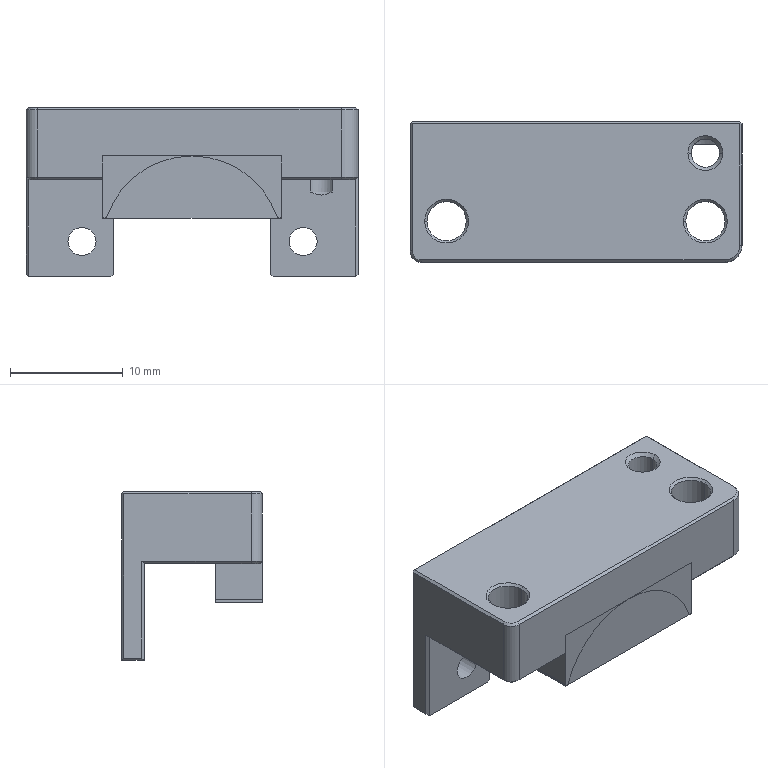NC program | NX | posted with a generic post | part box 29.5 x 12.5 x 15 mm
Whole program:
N10 G17 G21 G94 G90
(FLOOR_WALL_COPY_COPY , TOOL : D63)
N12 T03 M6
N14 G54
N16 G17 G0 G90 X-49.249 Y0. B0. C0. S6500 M3
N18 G43 Z30. H3
N20 Z7.
N22 G94 G1 Z4. F1250.
N24 X-46.249
N26 X46.249
N28 X49.249
N30 Z7.
N32 G0 Z30.
N34 X-49.249
N36 Z6.
N38 G1 Z3.
N40 X-46.249
N42 X46.249
N44 X49.249
N46 Z6.
N48 G0 Z30.
N50 X-49.249
N52 Z5.
N54 G1 Z2.
N56 X-46.249
N58 X46.249
N60 X49.249
N62 Z5.
N64 G0 Z30.
N66 X-49.249
N68 Z4.
N70 G1 Z1.
N72 X-46.249
N74 X46.249
N76 X49.249
N78 Z4.
N80 G0 Z30.
N82 X-49.249
N84 Z3.
N86 G1 Z0.
N88 X-46.249
N90 X46.249
N92 X49.249
N94 Z3.
N96 G0 Z30.
N98 M5
(FLOOR_WALL , TOOL : D6JING)
N100 T16 M6
N102 G54
N104 G17 G0 G90 X2.078 Y-12.25 B0. C0. S9500 M3
N106 G43 Z30. H16
N108 Z-0.443
N110 G94 G1 X0.52 Y-9.55 F1000.
N112 G3 X0. Y-9.25 R0.6
N114 G1 X-10.95 F2500.
N116 Y-9.05
N118 X-13.25
N120 G2 X-17.55 Y-4.75 R4.3
N122 G1 Y2.866
N124 X-15.834 Y1.15
N126 X-3.9
N128 Y9.25
N130 X3.9
N132 Y1.15
N134 X15.834
N136 X17.55 Y2.866
N138 Y-5.25
N140 G2 X13.75 Y-9.05 R3.8
N142 G1 X10.95
N144 Y-9.25
N146 X0.
N148 Y-6.25
N150 X-9.873
N152 G3 X-10.95 Y-6.05 R3.
N154 G1 X-13.25
N156 G2 X-14.55 Y-4.75 R1.3
N158 G1 Y-1.85
N160 X-3.9
N162 G3 X-0.9 Y1.15 R3.
N164 G1 Y6.25
N166 X0.9
N168 Y1.15
N170 G3 X3.9 Y-1.85 R3.
N172 G1 X14.55
N174 Y-5.25
N176 G2 X13.75 Y-6.05 R0.8
N178 G1 X10.95
N180 G3 X9.873 Y-6.25 R3.
N182 G1 X0.
N184 Y-3.55
N186 X-0.675
N188 G3 X0. Y-3.007 R5.7
N190 X0.675 Y-3.55 R5.7
N192 G1 X0.
N194 G3 X-0.52 Y-3.85 R0.6
N196 G1 Y-12.25
N198 G0 X2.078 Z-0.906
N200 G1 X0.52 Y-9.55 F1000.
N202 G3 X0. Y-9.25 R0.6
N204 G1 X-10.95 F2500.
N206 Y-9.05
N208 X-13.25
N210 G2 X-17.55 Y-4.75 R4.3
N212 G1 Y2.866
N214 X-15.834 Y1.15
N216 X-3.9
N218 Y9.25
N220 X3.9
N222 Y1.15
N224 X15.834
N226 X17.55 Y2.866
N228 Y-5.25
N230 G2 X13.75 Y-9.05 R3.8
N232 G1 X10.95
N234 Y-9.25
N236 X0.
N238 Y-6.25
N240 X-9.873
N242 G3 X-10.95 Y-6.05 R3.
N244 G1 X-13.25
N246 G2 X-14.55 Y-4.75 R1.3
N248 G1 Y-1.85
N250 X-3.9
N252 G3 X-0.9 Y1.15 R3.
N254 G1 Y6.25
N256 X0.9
N258 Y1.15
N260 G3 X3.9 Y-1.85 R3.
N262 G1 X14.55
N264 Y-5.25
N266 G2 X13.75 Y-6.05 R0.8
N268 G1 X10.95
N270 G3 X9.873 Y-6.25 R3.
N272 G1 X0.
N274 Y-3.55
N276 X-0.675
N278 G3 X0. Y-3.007 R5.7
N280 X0.675 Y-3.55 R5.7
N282 G1 X0.
N284 G3 X-0.52 Y-3.85 R0.6
N286 G1 Y-12.25
N288 G0 X2.078 Z-1.37
N290 G1 X0.52 Y-9.55 F1000.
N292 G3 X0. Y-9.25 R0.6
N294 G1 X-10.95 F2500.
N296 Y-9.05
N298 X-13.25
N300 G2 X-17.55 Y-4.75 R4.3
N302 G1 Y2.866
N304 X-15.834 Y1.15
N306 X-3.9
N308 Y9.25
N310 X3.9
N312 Y1.15
N314 X15.834
N316 X17.55 Y2.866
N318 Y-5.25
N320 G2 X13.75 Y-9.05 R3.8
N322 G1 X10.95
N324 Y-9.25
N326 X0.
N328 Y-6.25
N330 X-9.873
N332 G3 X-10.95 Y-6.05 R3.
N334 G1 X-13.25
N336 G2 X-14.55 Y-4.75 R1.3
N338 G1 Y-1.85
N340 X-3.9
N342 G3 X-0.9 Y1.15 R3.
N344 G1 Y6.25
N346 X0.9
N348 Y1.15
N350 G3 X3.9 Y-1.85 R3.
N352 G1 X14.55
N354 Y-5.25
N356 G2 X13.75 Y-6.05 R0.8
N358 G1 X10.95
N360 G3 X9.873 Y-6.25 R3.
N362 G1 X0.
N364 Y-3.55
N366 X-0.675
N368 G3 X0. Y-3.007 R5.7
N370 X0.675 Y-3.55 R5.7
N372 G1 X0.
N374 G3 X-0.52 Y-3.85 R0.6
N376 G1 Y-12.25
N378 G0 X2.078 Z-1.834
N380 G1 X0.52 Y-9.55 F1000.
N382 G3 X0. Y-9.25 R0.6
N384 G1 X-10.95 F2500.
N386 Y-9.05
N388 X-13.25
N390 G2 X-17.55 Y-4.75 R4.3
N392 G1 Y2.866
N394 X-15.834 Y1.15
N396 X-3.9
N398 Y9.25
N400 X3.9
N402 Y1.15
N404 X15.834
N406 X17.55 Y2.866
N408 Y-5.25
N410 G2 X13.75 Y-9.05 R3.8
N412 G1 X10.95
N414 Y-9.25
N416 X0.
N418 Y-6.25
N420 X-9.873
N422 G3 X-10.95 Y-6.05 R3.
N424 G1 X-13.25
N426 G2 X-14.55 Y-4.75 R1.3
N428 G1 Y-1.85
N430 X-3.9
N432 G3 X-0.9 Y1.15 R3.
N434 G1 Y6.25
N436 X0.9
N438 Y1.15
N440 G3 X3.9 Y-1.85 R3.
N442 G1 X14.55
N444 Y-5.25
N446 G2 X13.75 Y-6.05 R0.8
N448 G1 X10.95
N450 G3 X9.873 Y-6.25 R3.
N452 G1 X0.
N454 Y-3.55
N456 X-0.675
N458 G3 X0. Y-3.007 R5.7
N460 X0.675 Y-3.55 R5.7
N462 G1 X0.
N464 G3 X-0.52 Y-3.85 R0.6
N466 G1 Y-12.25
N468 G0 X2.078 Z-2.297
N470 G1 X0.52 Y-9.55 F1000.
N472 G3 X0. Y-9.25 R0.6
N474 G1 X-10.95 F2500.
N476 Y-9.05
N478 X-13.25
N480 G2 X-17.55 Y-4.75 R4.3
N482 G1 Y2.866
N484 X-15.834 Y1.15
N486 X-3.9
N488 Y9.25
N490 X3.9
N492 Y1.15
N494 X15.834
N496 X17.55 Y2.866
N498 Y-5.25
N500 G2 X13.75 Y-9.05 R3.8
N502 G1 X10.95
N504 Y-9.25
N506 X0.
N508 Y-6.25
N510 X-9.873
N512 G3 X-10.95 Y-6.05 R3.
N514 G1 X-13.25
N516 G2 X-14.55 Y-4.75 R1.3
N518 G1 Y-1.85
N520 X-3.9
N522 G3 X-0.9 Y1.15 R3.
N524 G1 Y6.25
N526 X0.9
N528 Y1.15
N530 G3 X3.9 Y-1.85 R3.
N532 G1 X14.55
N534 Y-5.25
N536 G2 X13.75 Y-6.05 R0.8
N538 G1 X10.95
N540 G3 X9.873 Y-6.25 R3.
N542 G1 X0.
N544 Y-3.55
N546 X-0.675
N548 G3 X0. Y-3.007 R5.7
N550 X0.675 Y-3.55 R5.7
N552 G1 X0.
N554 G3 X-0.52 Y-3.85 R0.6
N556 G1 Y-12.25
N558 G0 X2.078 Z-2.761
N560 G1 X0.52 Y-9.55 F1000.
N562 G3 X0. Y-9.25 R0.6
N564 G1 X-10.95 F2500.
N566 Y-9.05
N568 X-13.25
N570 G2 X-17.55 Y-4.75 R4.3
N572 G1 Y2.866
N574 X-15.834 Y1.15
N576 X-3.9
N578 Y9.25
N580 X3.9
N582 Y1.15
N584 X15.834
N586 X17.55 Y2.866
N588 Y-5.25
N590 G2 X13.75 Y-9.05 R3.8
N592 G1 X10.95
N594 Y-9.25
N596 X0.
N598 Y-6.25
N600 X-9.873
N602 G3 X-10.95 Y-6.05 R3.
N604 G1 X-13.25
N606 G2 X-14.55 Y-4.75 R1.3
N608 G1 Y-1.85
N610 X-3.9
N612 G3 X-0.9 Y1.15 R3.
N614 G1 Y6.25
N616 X0.9
N618 Y1.15
N620 G3 X3.9 Y-1.85 R3.
N622 G1 X14.55
N624 Y-5.25
N626 G2 X13.75 Y-6.05 R0.8
N628 G1 X10.95
N630 G3 X9.873 Y-6.25 R3.
N632 G1 X0.
N634 Y-3.55
N636 X-0.675
N638 G3 X0. Y-3.007 R5.7
N640 X0.675 Y-3.55 R5.7
N642 G1 X0.
N644 G3 X-0.52 Y-3.85 R0.6
N646 G1 Y-12.25
N648 G0 X2.078 Z-3.225
N650 G1 X0.52 Y-9.55 F1000.
N652 G3 X0. Y-9.25 R0.6
N654 G1 X-10.95 F2500.
N656 Y-9.05
N658 X-13.25
N660 G2 X-17.55 Y-4.75 R4.3
N662 G1 Y2.866
N664 X-15.834 Y1.15
N666 X-3.9
N668 Y9.25
N670 X3.9
N672 Y1.15
N674 X15.834
N676 X17.55 Y2.866
N678 Y-5.25
N680 G2 X13.75 Y-9.05 R3.8
N682 G1 X10.95
N684 Y-9.25
N686 X0.
N688 Y-6.25
N690 X-9.873
N692 G3 X-10.95 Y-6.05 R3.
N694 G1 X-13.25
N696 G2 X-14.55 Y-4.75 R1.3
N698 G1 Y-1.85
N700 X-3.9
N702 G3 X-0.9 Y1.15 R3.
N704 G1 Y6.25
N706 X0.9
N708 Y1.15
N710 G3 X3.9 Y-1.85 R3.
N712 G1 X14.55
N714 Y-5.25
N716 G2 X13.75 Y-6.05 R0.8
N718 G1 X10.95
N720 G3 X9.873 Y-6.25 R3.
N722 G1 X0.
N724 Y-3.55
N726 X-0.675
N728 G3 X0. Y-3.007 R5.7
N730 X0.675 Y-3.55 R5.7
N732 G1 X0.
N734 G3 X-0.52 Y-3.85 R0.6
N736 G1 Y-12.25
N738 G0 X2.078 Z-3.688
N740 G1 X0.52 Y-9.55 F1000.
N742 G3 X0. Y-9.25 R0.6
N744 G1 X-10.95 F2500.
N746 Y-9.05
N748 X-13.25
N750 G2 X-17.55 Y-4.75 R4.3
N752 G1 Y2.866
N754 X-15.834 Y1.15
N756 X-3.9
N758 Y9.25
N760 X3.9
N762 Y1.15
N764 X15.834
N766 X17.55 Y2.866
N768 Y-5.25
N770 G2 X13.75 Y-9.05 R3.8
N772 G1 X10.95
N774 Y-9.25
N776 X0.
N778 Y-6.25
N780 X-9.873
N782 G3 X-10.95 Y-6.05 R3.
N784 G1 X-13.25
N786 G2 X-14.55 Y-4.75 R1.3
N788 G1 Y-1.85
N790 X-3.9
N792 G3 X-0.9 Y1.15 R3.
N794 G1 Y6.25
N796 X0.9
N798 Y1.15
N800 G3 X3.9 Y-1.85 R3.
N802 G1 X14.55
N804 Y-5.25
N806 G2 X13.75 Y-6.05 R0.8
N808 G1 X10.95
N810 G3 X9.873 Y-6.25 R3.
N812 G1 X0.
N814 Y-3.55
N816 X-0.675
N818 G3 X0. Y-3.007 R5.7
N820 X0.675 Y-3.55 R5.7
N822 G1 X0.
N824 G3 X-0.52 Y-3.85 R0.6
N826 G1 Y-12.25
N828 G0 X2.078 Z-4.152
N830 G1 X0.52 Y-9.55 F1000.
N832 G3 X0. Y-9.25 R0.6
N834 G1 X-10.95 F2500.
N836 Y-9.05
N838 X-13.25
N840 G2 X-17.55 Y-4.75 R4.3
N842 G1 Y2.866
N844 X-15.834 Y1.15
N846 X-3.9
N848 Y9.25
N850 X3.9
N852 Y1.15
N854 X15.834
N856 X17.55 Y2.866
N858 Y-5.25
N860 G2 X13.75 Y-9.05 R3.8
N862 G1 X10.95
N864 Y-9.25
N866 X0.
N868 Y-6.25
N870 X-9.873
N872 G3 X-10.95 Y-6.05 R3.
N874 G1 X-13.25
N876 G2 X-14.55 Y-4.75 R1.3
N878 G1 Y-1.85
N880 X-3.9
N882 G3 X-0.9 Y1.15 R3.
N884 G1 Y6.25
N886 X0.9
N888 Y1.15
N890 G3 X3.9 Y-1.85 R3.
N892 G1 X14.55
N894 Y-5.25
N896 G2 X13.75 Y-6.05 R0.8
N898 G1 X10.95
N900 G3 X9.873 Y-6.25 R3.
N902 G1 X0.
N904 Y-3.55
N906 X-0.675
N908 G3 X0. Y-3.007 R5.7
N910 X0.675 Y-3.55 R5.7
N912 G1 X0.
N914 G3 X-0.52 Y-3.85 R0.6
N916 G1 Y-12.25
N918 G0 X2.078 Z-4.615
N920 G1 X0.52 Y-9.55 F1000.
N922 G3 X0. Y-9.25 R0.6
N924 G1 X-10.95 F2500.
N926 Y-9.05
N928 X-13.25
N930 G2 X-17.55 Y-4.75 R4.3
N932 G1 Y2.866
N934 X-15.834 Y1.15
N936 X-3.9
N938 Y9.25
N940 X3.9
N942 Y1.15
N944 X15.834
N946 X17.55 Y2.866
N948 Y-5.25
N950 G2 X13.75 Y-9.05 R3.8
N952 G1 X10.95
N954 Y-9.25
N956 X0.
N958 Y-6.25
N960 X-9.873
N962 G3 X-10.95 Y-6.05 R3.
N964 G1 X-13.25
N966 G2 X-14.55 Y-4.75 R1.3
N968 G1 Y-1.85
N970 X-3.9
N972 G3 X-0.9 Y1.15 R3.
N974 G1 Y6.25
N976 X0.9
N978 Y1.15
N980 G3 X3.9 Y-1.85 R3.
N982 G1 X14.55
N984 Y-5.25
N986 G2 X13.75 Y-6.05 R0.8
N988 G1 X10.95
N990 G3 X9.873 Y-6.25 R3.
N992 G1 X0.
N994 Y-3.55
N996 X-0.675
N998 G3 X0. Y-3.007 R5.7
N1000 X0.675 Y-3.55 R5.7
N1002 G1 X0.
N1004 G3 X-0.52 Y-3.85 R0.6
N1006 G1 Y-12.25
N1008 G0 X2.078 Z-5.079
N1010 G1 X0.52 Y-9.55 F1000.
N1012 G3 X0. Y-9.25 R0.6
N1014 G1 X-10.95 F2500.
N1016 Y-9.05
N1018 X-13.25
N1020 G2 X-17.55 Y-4.75 R4.3
N1022 G1 Y2.866
N1024 X-15.834 Y1.15
N1026 X-3.9
N1028 Y9.25
N1030 X3.9
N1032 Y1.15
N1034 X15.834
N1036 X17.55 Y2.866
N1038 Y-5.25
N1040 G2 X13.75 Y-9.05 R3.8
N1042 G1 X10.95
N1044 Y-9.25
N1046 X0.
N1048 Y-6.25
N1050 X-9.873
N1052 G3 X-10.95 Y-6.05 R3.
N1054 G1 X-13.25
N1056 G2 X-14.55 Y-4.75 R1.3
N1058 G1 Y-1.85
N1060 X-3.9
N1062 G3 X-0.9 Y1.15 R3.
N1064 G1 Y6.25
N1066 X0.9
N1068 Y1.15
N1070 G3 X3.9 Y-1.85 R3.
N1072 G1 X14.55
N1074 Y-5.25
N1076 G2 X13.75 Y-6.05 R0.8
N1078 G1 X10.95
N1080 G3 X9.873 Y-6.25 R3.
N1082 G1 X0.
N1084 Y-3.55
N1086 X-0.675
N1088 G3 X0. Y-3.007 R5.7
N1090 X0.675 Y-3.55 R5.7
N1092 G1 X0.
N1094 G3 X-0.52 Y-3.85 R0.6
N1096 G1 Y-12.25
N1098 G0 Z30.
N1100 X-2.136 Y12.35
N1102 Z-5.568
N1104 G1 X-0.52 Y9.55 F1000.
N1106 G3 X0. Y9.25 R0.6
N1108 G1 X3.9 F2500.
N1110 Y1.15
N1112 X15.834
N1114 X17.55 Y2.866
N1116 Y-5.25
N1118 G2 X13.75 Y-9.05 R3.8
N1120 G1 X11.05
N1122 Y-1.85
N1124 X14.05
N1126 X14.55
N1128 Y-5.25
N1130 G2 X14.05 Y-5.992 R0.8
N1132 G1 Y-1.85
N1134 X11.05
N1136 Y1.05
N1138 X-11.05
N1140 Y-9.05
N1142 X-13.25
N1144 G2 X-17.55 Y-4.75 R4.3
N1146 G1 Y2.866
N1148 X-15.834 Y1.15
N1150 X-14.05
N1152 Y-1.85
N1154 Y-5.775
N1156 G2 X-14.55 Y-4.75 R1.3
N1158 G1 Y-1.85
N1160 X-14.05
N1162 Y1.15
N1164 X-3.9
N1166 Y9.25
N1168 X0.
N1170 Y6.25
N1172 X0.9
N1174 Y4.05
N1176 X-0.9
N1178 Y6.25
N1180 X0.
N1182 G3 X0.52 Y6.55 R0.6
N1184 G1 Y12.25
N1186 G0 X-2.136 Y12.35 Z-6.056
N1188 G1 X-0.52 Y9.55 F1000.
N1190 G3 X0. Y9.25 R0.6
N1192 G1 X3.9 F2500.
N1194 Y1.15
N1196 X15.834
N1198 X17.55 Y2.866
N1200 Y-5.25
N1202 G2 X13.75 Y-9.05 R3.8
N1204 G1 X11.05
N1206 Y-1.85
N1208 X14.05
N1210 X14.55
N1212 Y-5.25
N1214 G2 X14.05 Y-5.992 R0.8
N1216 G1 Y-1.85
N1218 X11.05
N1220 Y1.05
N1222 X-11.05
N1224 Y-9.05
N1226 X-13.25
N1228 G2 X-17.55 Y-4.75 R4.3
N1230 G1 Y2.866
N1232 X-15.834 Y1.15
N1234 X-14.05
N1236 Y-1.85
N1238 Y-5.775
N1240 G2 X-14.55 Y-4.75 R1.3
N1242 G1 Y-1.85
N1244 X-14.05
N1246 Y1.15
N1248 X-3.9
N1250 Y9.25
N1252 X0.
N1254 Y6.25
N1256 X0.9
N1258 Y4.05
N1260 X-0.9
N1262 Y6.25
N1264 X0.
N1266 G3 X0.52 Y6.55 R0.6
N1268 G1 Y12.25
N1270 G0 X-2.136 Y12.35 Z-6.545
N1272 G1 X-0.52 Y9.55 F1000.
N1274 G3 X0. Y9.25 R0.6
N1276 G1 X3.9 F2500.
N1278 Y1.15
N1280 X15.834
N1282 X17.55 Y2.866
N1284 Y-5.25
N1286 G2 X13.75 Y-9.05 R3.8
N1288 G1 X11.05
N1290 Y-1.85
N1292 X14.05
N1294 X14.55
N1296 Y-5.25
N1298 G2 X14.05 Y-5.992 R0.8
N1300 G1 Y-1.85
N1302 X11.05
N1304 Y1.05
N1306 X-11.05
N1308 Y-9.05
N1310 X-13.25
N1312 G2 X-17.55 Y-4.75 R4.3
N1314 G1 Y2.866
N1316 X-15.834 Y1.15
N1318 X-14.05
N1320 Y-1.85
N1322 Y-5.775
N1324 G2 X-14.55 Y-4.75 R1.3
N1326 G1 Y-1.85
N1328 X-14.05
N1330 Y1.15
N1332 X-3.9
N1334 Y9.25
N1336 X0.
N1338 Y6.25
N1340 X0.9
N1342 Y4.05
N1344 X-0.9
N1346 Y6.25
N1348 X0.
N1350 G3 X0.52 Y6.55 R0.6
N1352 G1 Y12.25
N1354 G0 X-2.136 Y12.35 Z-7.034
N1356 G1 X-0.52 Y9.55 F1000.
N1358 G3 X0. Y9.25 R0.6
N1360 G1 X3.9 F2500.
N1362 Y1.15
N1364 X15.834
N1366 X17.55 Y2.866
N1368 Y-5.25
N1370 G2 X13.75 Y-9.05 R3.8
N1372 G1 X11.05
N1374 Y-1.85
N1376 X14.05
N1378 X14.55
N1380 Y-5.25
N1382 G2 X14.05 Y-5.992 R0.8
N1384 G1 Y-1.85
N1386 X11.05
N1388 Y1.05
N1390 X-11.05
N1392 Y-9.05
N1394 X-13.25
N1396 G2 X-17.55 Y-4.75 R4.3
N1398 G1 Y2.866
N1400 X-15.834 Y1.15
N1402 X-14.05
N1404 Y-1.85
N1406 Y-5.775
N1408 G2 X-14.55 Y-4.75 R1.3
N1410 G1 Y-1.85
N1412 X-14.05
N1414 Y1.15
N1416 X-3.9
N1418 Y9.25
N1420 X0.
N1422 Y6.25
N1424 X0.9
N1426 Y4.05
N1428 X-0.9
N1430 Y6.25
N1432 X0.
N1434 G3 X0.52 Y6.55 R0.6
N1436 G1 Y12.25
N1438 G0 X-2.136 Y12.35 Z-7.523
N1440 G1 X-0.52 Y9.55 F1000.
N1442 G3 X0. Y9.25 R0.6
N1444 G1 X3.9 F2500.
N1446 Y1.15
N1448 X15.834
N1450 X17.55 Y2.866
N1452 Y-5.25
N1454 G2 X13.75 Y-9.05 R3.8
N1456 G1 X11.05
N1458 Y-1.85
N1460 X14.05
N1462 X14.55
N1464 Y-5.25
N1466 G2 X14.05 Y-5.992 R0.8
N1468 G1 Y-1.85
N1470 X11.05
N1472 Y1.05
N1474 X-11.05
N1476 Y-9.05
N1478 X-13.25
N1480 G2 X-17.55 Y-4.75 R4.3
N1482 G1 Y2.866
N1484 X-15.834 Y1.15
N1486 X-14.05
N1488 Y-1.85
N1490 Y-5.775
N1492 G2 X-14.55 Y-4.75 R1.3
N1494 G1 Y-1.85
N1496 X-14.05
N1498 Y1.15
N1500 X-3.9
N1502 Y9.25
N1504 X0.
N1506 Y6.25
N1508 X0.9
N1510 Y4.05
N1512 X-0.9
N1514 Y6.25
N1516 X0.
N1518 G3 X0.52 Y6.55 R0.6
N1520 G1 Y12.25
N1522 G0 X-2.136 Y12.35 Z-8.011
N1524 G1 X-0.52 Y9.55 F1000.
N1526 G3 X0. Y9.25 R0.6
N1528 G1 X3.9 F2500.
N1530 Y1.15
N1532 X15.834
N1534 X17.55 Y2.866
N1536 Y-5.25
N1538 G2 X13.75 Y-9.05 R3.8
N1540 G1 X11.05
N1542 Y-1.85
N1544 X14.05
N1546 X14.55
N1548 Y-5.25
N1550 G2 X14.05 Y-5.992 R0.8
N1552 G1 Y-1.85
N1554 X11.05
N1556 Y1.05
N1558 X-11.05
N1560 Y-9.05
N1562 X-13.25
N1564 G2 X-17.55 Y-4.75 R4.3
N1566 G1 Y2.866
N1568 X-15.834 Y1.15
N1570 X-14.05
N1572 Y-1.85
N1574 Y-5.775
N1576 G2 X-14.55 Y-4.75 R1.3
N1578 G1 Y-1.85
N1580 X-14.05
N1582 Y1.15
N1584 X-3.9
N1586 Y9.25
N1588 X0.
N1590 Y6.25
N1592 X0.9
N1594 Y4.05
N1596 X-0.9
N1598 Y6.25
N1600 X0.
N1602 G3 X0.52 Y6.55 R0.6
N1604 G1 Y12.25
N1606 G0 X-2.136 Y12.35 Z-8.5
N1608 G1 X-0.52 Y9.55 F1000.
N1610 G3 X0. Y9.25 R0.6
N1612 G1 X3.9 F2500.
N1614 Y1.15
N1616 X15.834
N1618 X17.55 Y2.866
N1620 Y-5.25
N1622 G2 X13.75 Y-9.05 R3.8
N1624 G1 X11.05
N1626 Y-1.85
N1628 X14.05
N1630 X14.55
N1632 Y-5.25
N1634 G2 X14.05 Y-5.992 R0.8
N1636 G1 Y-1.85
N1638 X11.05
N1640 Y1.05
N1642 X-11.05
N1644 Y-9.05
N1646 X-13.25
N1648 G2 X-17.55 Y-4.75 R4.3
N1650 G1 Y2.866
N1652 X-15.834 Y1.15
N1654 X-14.05
N1656 Y-1.85
N1658 Y-5.775
N1660 G2 X-14.55 Y-4.75 R1.3
N1662 G1 Y-1.85
N1664 X-14.05
N1666 Y1.15
N1668 X-3.9
N1670 Y9.25
N1672 X0.
N1674 Y6.25
N1676 X0.9
N1678 Y4.05
N1680 X-0.9
N1682 Y6.25
N1684 X0.
N1686 G3 X0.52 Y6.55 R0.6
N1688 G1 Y12.25
N1690 G0 X-2.136 Y12.35 Z-9.
N1692 G1 X-0.52 Y9.55 F1000.
N1694 G3 X0. Y9.25 R0.6
N1696 G1 X3.9 F2500.
N1698 Y1.05
N1700 X-3.9
N1702 Y9.25
N1704 X0.
N1706 Y6.25
N1708 X0.9
N1710 Y4.05
N1712 X-0.9
N1714 Y6.25
N1716 X0.
N1718 G3 X0.52 Y6.55 R0.6
N1720 G1 Y12.25
N1722 G0 X-2.136 Y12.35 Z-9.5
N1724 G1 X-0.52 Y9.55 F1000.
N1726 G3 X0. Y9.25 R0.6
N1728 G1 X3.9 F2500.
N1730 Y1.05
N1732 X-3.9
N1734 Y9.25
N1736 X0.
N1738 Y6.25
N1740 X0.9
N1742 Y4.05
N1744 X-0.9
N1746 Y6.25
N1748 X0.
N1750 G3 X0.52 Y6.55 R0.6
N1752 G1 Y12.25
N1754 G0 Z30.
(FLOOR_WALL_COPY_1 , TOOL : D6JING)
N1756 X0.924 Y-10.25
N1758 Z-4.179
N1760 G1 Z-5.179 F1000.
N1762 X0.52 Y-9.55
N1764 G3 X0. Y-9.25 R0.6
N1766 G1 X-10.95
N1768 Y0.95
N1770 X10.95
N1772 Y-9.25
N1774 X0.
N1776 Y-6.25
N1778 X-7.95
N1780 Y-2.05
N1782 X7.95
N1784 Y-6.25
N1786 X0.
N1788 G3 X-0.52 Y-6.55 R0.6
N1790 G1 Z-4.179
N1792 G0 Z30.
N1794 X-0.924 Y10.25
N1796 Z-8.6
N1798 G1 Z-9.6
N1800 X-0.52 Y9.55
N1802 G3 X0. Y9.25 R0.6
N1804 G1 X3.7
N1806 Y1.25
N1808 X-3.7
N1810 Y9.25
N1812 X0.
N1814 Y6.25
N1816 X0.7
N1818 Y4.25
N1820 X-0.7
N1822 Y6.25
N1824 X0.
N1826 G3 X0.52 Y6.55 R0.6
N1828 G1 Z-8.6
N1830 G0 Z-6.5
N1832 G1 X-2.868 Y10.25 F8000.
N1834 G0 Z-8.6
N1836 G1 Z-9.6 F1000.
N1838 X-3.7 Y9.77
N1840 G3 X-4. Y9.25 R0.6
N1842 G1 Y0.95
N1844 X4.
N1846 Y9.25
N1848 G3 X3.7 Y9.77 R0.6
N1850 G1 X2.868 Y10.25
N1852 Z-8.6
N1854 G0 Z30.
(FLOOR_WALL_COPY_1_COPY , TOOL : D6JING)
N1856 X-18.55 Y-4.374
N1858 Z-7.6
N1860 G1 Z-8.6
N1862 X-17.85 Y-3.97
N1864 G3 X-17.55 Y-3.45 R0.6
N1866 G1 Y2.442
N1868 X-16.046 Y0.938
N1870 G3 X-15.834 Y0.85 R0.3
N1872 G1 X-11.35
N1874 Y-9.05
N1876 X-13.25
N1878 G2 X-17.55 Y-4.75 R4.3
N1880 G1 Y-3.45
N1882 X-14.55
N1884 Y-2.15
N1886 X-14.35
N1888 Y-5.443
N1890 G2 X-14.55 Y-4.75 R1.3
N1892 G1 Y-3.45
N1894 G3 X-14.85 Y-2.93 R0.6
N1896 G1 Z-7.6
N1898 G0 Z-5.5
N1900 G1 X-12.182 Y-10.05 F8000.
N1902 G0 Z-7.6
N1904 G1 Z-8.6 F1000.
N1906 X-11.35 Y-9.57
N1908 G3 X-11.05 Y-9.05 R0.6
N1910 G1 Y1.05
N1912 X-4.
N1914 G3 X-3.48 Y1.35 R0.6
N1916 G1 X-3.85 Y1.11
N1918 X-3.894 Y1.141
N1920 X-3.946 Y1.155
N1922 X-4. Y1.15
N1924 X-15.834
N1926 X-17.55 Y2.866
N1928 G3 X-18.13 Y3.021 R0.6
N1930 G1 X-18.85 Y2.828
N1932 Z-7.6
N1934 G0 Z30.
N1936 X18.55 Y-2.776
N1938 Z-7.6
N1940 G1 Z-8.6
N1942 X17.85 Y-3.18
N1944 G3 X17.55 Y-3.7 R0.6
N1946 G1 Y-5.25
N1948 G2 X13.75 Y-9.05 R3.8
N1950 G1 X11.35
N1952 Y0.85
N1954 X15.834
N1956 G3 X16.046 Y0.938 R0.3
N1958 G1 X17.55 Y2.442
N1960 Y-3.7
N1962 X14.55
N1964 Y-5.25
N1966 G2 X14.35 Y-5.779 R0.8
N1968 G1 Y-2.15
N1970 X14.55
N1972 Y-3.7
N1974 G3 X14.85 Y-4.22 R0.6
N1976 G1 Z-7.6
N1978 G0 Z-5.5
N1980 G1 X18.85 Y2.816 F8000.
N1982 G0 Z-7.6
N1984 G1 Z-8.6 F1000.
N1986 X18.12 Y3.011
N1988 G3 X17.54 Y2.856 R0.6
N1990 G1 X15.834 Y1.15
N1992 X4.
N1994 X3.946 Y1.155
N1996 X3.894 Y1.141
N1998 X3.85 Y1.11
N2000 X3.48 Y1.35
N2002 G3 X4. Y1.05 R0.6
N2004 G1 X11.05
N2006 Y-9.05
N2008 G3 X11.35 Y-9.57 R0.6
N2010 G1 X12.182 Y-10.05
N2012 Z-7.6
N2014 G0 Z30.
(ZLEVEL_PROFILE_1_COPY_COPY , TOOL : D6JING)
N2016 X-3.781 Y1.25
N2018 Z1.
N2020 G1 Z-8.6
N2022 X-6.649
N2024 X-6.662 Y1.269
N2026 G2 X-7. Y1.25 R3.
N2028 G1 X-14.55
N2030 G2 X-16.721 Y2.179 R3.001
N2032 G1 X-16.871 Y2.329
N2034 G2 X-17.102 Y2.587 R3.
N2036 G1 X-17.118 Y2.575
N2038 X-19.208 Y4.668
N2040 G3 X-19.788 Y4.824 R0.6
N2042 G1 X-20.054 Y4.753
N2044 Z-7.6
N2046 G0 Z30.
N2048 X19.959 Y4.613
N2050 Z-7.6
N2052 G1 Z-8.6
N2054 X19.657 Y4.693
N2056 G3 X19.078 Y4.538 R0.6
N2058 G1 X16.871 Y2.329
N2060 X16.671 Y2.129
N2062 G2 X14.55 Y1.25 R3.
N2064 G1 X7.218
N2066 X6.875 Y1.248
N2068 X4.039
N2070 X3.738 Y1.25
N2072 G3 X3.217 Y0.952 R0.6
N2074 G1 Z-7.6
N2076 G0 Z30.
N2078 M5
(ZLEVEL_PROFILE_COPY_COPY_COPY_1_COPY_COPY , TOOL : D2)
N2080 T18 M6
N2082 G54
N2084 G17 G0 G90 X-5.6 Y1.513 B0. C0. S9500 M3
N2086 G43 Z30. H18
N2088 Z-8.8
N2090 G94 G1 X-5.9 Y1.34 F1000.
N2092 G3 X-6. Y1.166 R0.2
N2094 G1 Y-1.05
N2096 X-3.784
N2098 G3 X-3.61 Y-0.95 R0.2
N2100 G1 X-3.437 Y-0.65
N2102 G0 X-5.6 Y1.513 Z-9.
N2104 G1 X-5.9 Y1.34
N2106 G3 X-6. Y1.166 R0.2
N2108 G1 Y-1.05
N2110 X-3.784
N2112 G3 X-3.61 Y-0.95 R0.2
N2114 G1 X-3.437 Y-0.65
N2116 G0 X-5.6 Y1.513 Z-9.2
N2118 G1 X-5.9 Y1.34
N2120 G3 X-6. Y1.166 R0.2
N2122 G1 Y-1.05
N2124 X-3.784
N2126 G3 X-3.61 Y-0.95 R0.2
N2128 G1 X-3.437 Y-0.65
N2130 G0 X-5.6 Y1.513 Z-9.4
N2132 G1 X-5.9 Y1.34
N2134 G3 X-6. Y1.166 R0.2
N2136 G1 Y-1.05
N2138 X-3.784
N2140 G3 X-3.61 Y-0.95 R0.2
N2142 G1 X-3.437 Y-0.65
N2144 G0 X-5.6 Y1.513 Z-9.6
N2146 G1 X-5.9 Y1.34
N2148 G3 X-6. Y1.166 R0.2
N2150 G1 Y-1.05
N2152 X-3.784
N2154 G3 X-3.61 Y-0.95 R0.2
N2156 G1 X-3.437 Y-0.65
N2158 G0 Z30.
N2160 X3.437
N2162 Z-8.8
N2164 G1 X3.61 Y-0.95
N2166 G3 X3.784 Y-1.05 R0.2
N2168 G1 X6.
N2170 Y1.166
N2172 G3 X5.9 Y1.34 R0.2
N2174 G1 X5.6 Y1.513
N2176 G0 X3.437 Y-0.65 Z-9.
N2178 G1 X3.61 Y-0.95
N2180 G3 X3.784 Y-1.05 R0.2
N2182 G1 X6.
N2184 Y1.166
N2186 G3 X5.9 Y1.34 R0.2
N2188 G1 X5.6 Y1.513
N2190 G0 X3.437 Y-0.65 Z-9.2
N2192 G1 X3.61 Y-0.95
N2194 G3 X3.784 Y-1.05 R0.2
N2196 G1 X6.
N2198 Y1.166
N2200 G3 X5.9 Y1.34 R0.2
N2202 G1 X5.6 Y1.513
N2204 G0 X3.437 Y-0.65 Z-9.4
N2206 G1 X3.61 Y-0.95
N2208 G3 X3.784 Y-1.05 R0.2
N2210 G1 X6.
N2212 Y1.166
N2214 G3 X5.9 Y1.34 R0.2
N2216 G1 X5.6 Y1.513
N2218 G0 X3.437 Y-0.65 Z-9.6
N2220 G1 X3.61 Y-0.95
N2222 G3 X3.784 Y-1.05 R0.2
N2224 G1 X6.
N2226 Y1.166
N2228 G3 X5.9 Y1.34 R0.2
N2230 G1 X5.6 Y1.513
N2232 G0 Z30.
N2234 M5
(11_COPY_COPY_1 , TOOL : D6A45)
N2236 T01 M6
N2238 G54
N2240 G17 G0 G90 X6.279 Y8.202 B0. C0. S9500 M3
N2242 G43 Z30. H1
N2244 Z2.
N2246 G94 G1 Z-1. F1000.
N2248 X6.679 Y7.509
N2250 G3 X7.199 Y7.209 R0.6
N2252 G1 X14.555
N2254 G2 X15.509 Y6.255 R0.954
N2256 G1 Y4.244
N2258 G2 X14.556 Y3.291 R0.953
N2260 G1 X7.199
N2262 G2 X6.241 Y4.249 R0.958
N2264 G1 Y6.251
N2266 G2 X7.199 Y7.209 R0.958
N2268 G3 X7.719 Y7.509 R0.6
N2270 G1 X8.238 Y8.409
N2272 Z2.
N2274 G0 Z30.
N2276 X-15.475 Y8.202
N2278 Z2.
N2280 G1 Z-1.
N2282 X-15.075 Y7.509
N2284 G3 X-14.555 Y7.209 R0.6
N2286 G1 X-7.199
N2288 G2 X-6.241 Y6.251 R0.958
N2290 G1 Y4.249
N2292 G2 X-7.199 Y3.291 R0.958
N2294 G1 X-14.556
N2296 G2 X-15.509 Y4.244 R0.953
N2298 G1 Y6.255
N2300 G2 X-14.555 Y7.209 R0.954
N2302 G3 X-14.035 Y7.509 R0.6
N2304 G1 X-13.516 Y8.409
N2306 Z2.
N2308 G0 Z30.
(11_COPY_COPY_1_COPY , TOOL : D6A45)
N2310 X-3.839 Y8.909
N2312 Z-8.1
N2314 G1 Z-11.1
N2316 X-4.294 Y7.859
N2318 G3 X-4.034 Y7.709 R0.3
N2320 G1 X4.034
N2322 G3 X4.294 Y7.859 R0.3
N2324 G1 X3.842 Y8.909
N2326 Z-8.1
N2328 G0 Z30.
N2330 X18.751 Y3.382
N2332 Z-8.1
N2334 G1 Z-11.1
N2336 X17.309 Y2.549
N2338 G3 X17.009 Y2.029 R0.6
N2340 G1 Y-5.263
N2342 G2 X13.76 Y-8.509 R3.259
N2344 G1 X10.369
N2346 G3 X9.85 Y-8.809 R0.6
N2348 G1 X9.024 Y-10.238
N2350 Z-8.1
N2352 G0 Z30.
N2354 X-9.021 Y-10.239
N2356 Z-8.1
N2358 G1 Z-11.1
N2360 X-9.847 Y-8.809
N2362 G3 X-10.366 Y-8.509 R0.6
N2364 G1 X-13.26
N2366 G2 X-17.009 Y-4.76 R3.759
N2368 G1 Y2.033
N2370 G3 X-17.309 Y2.553 R0.6
N2372 G1 X-18.742 Y3.38
N2374 Z-8.1
N2376 G0 Z30.
N2378 M5
(刀补16 , TOOL : D6JING)
N2380 T16 M6
N2382 G54
N2384 G17 G0 G90 X-12.206 Y-10.174 B0. C0. S9500 M3
N2386 G43 Z30. H16
N2388 Z-7.6
N2390 G94 G1 Z-8.6 F1000.
N2392 G41 X-11.044 Y-10.002 D16
N2394 X-11.049 Y-9.402
N2396 X-11.051 Y-9.052
N2398 Y-6.262
N2400 X-11.05 Y-6.251
N2402 Y-2.05
N2404 X-11.052 Y-1.699
N2406 X-11.05 Y1.102
N2408 X-11.079 Y1.15
N2410 G40
N2412 X-12.251 Y-0.05
N2414 Z-7.6
N2416 G0 Z30.
N2418 X12.25
N2420 Z-7.6
N2422 G1 Z-8.6
N2424 G41 X11.079 Y1.15
N2426 X11.05 Y1.102
N2428 Y-2.05
N2430 Y-5.901
N2432 X11.051 Y-6.251
N2434 Y-9.052
N2436 X11.049 Y-9.402
N2438 X11.047 Y-10.002
N2440 G40
N2442 X12.207 Y-10.173
N2444 Z-7.6
N2446 G0 Z30.
N2448 M5
N2450 M2